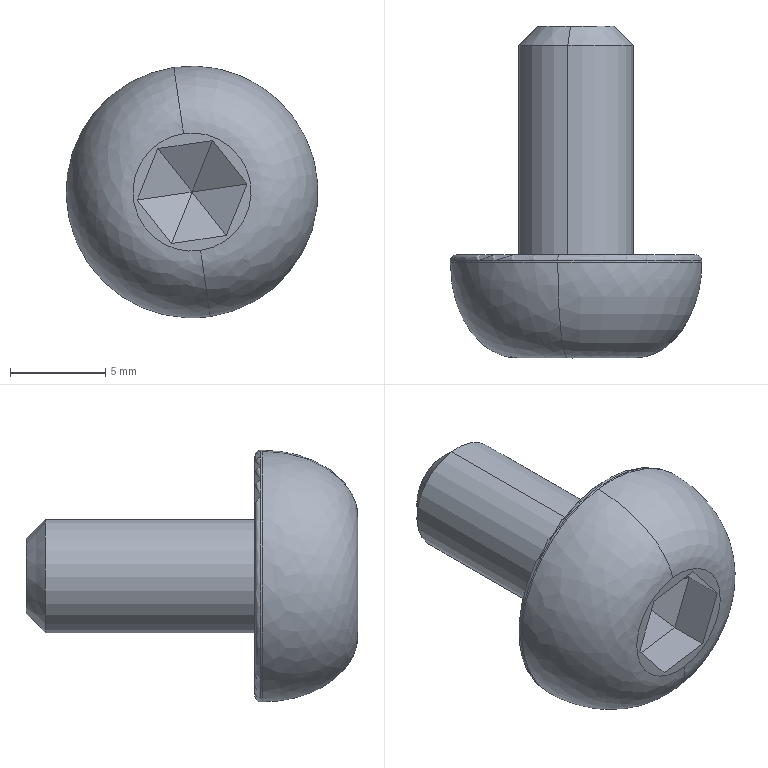Part | SolidWorks | features BaseBody 1 | 1 solid | 25 faces | box 13.2 x 17.4 x 13.2 mm | volume 875.551 mm3 | plane 15 | cylinder 4 | cone 2 | torus 2 | spline 2 | commonest cylinder face diameters 6 x2 13.2 x2
STEP:
#1=CARTESIAN_POINT('',(-484.979,-95.35,173.865));
#2=VERTEX_POINT('',#1);
#3=CARTESIAN_POINT('',(-485.556,-95.35,177.823));
#4=VERTEX_POINT('',#3);
#5=CARTESIAN_POINT('',(-485.268,-95.35,175.844));
#6=DIRECTION('',(0.,1.,0.));
#7=DIRECTION('',(0.1444,0.,-0.9895));
#8=AXIS2_PLACEMENT_3D('',#5,#6,#7);
#9=CIRCLE('',#8,2.);
#10=EDGE_CURVE('',#2,#4,#9,.T.);
#11=ORIENTED_EDGE('',*,*,#10,.F.);
#12=CARTESIAN_POINT('',(-484.835,-96.35,172.876));
#13=VERTEX_POINT('',#12);
#14=CARTESIAN_POINT('',(-484.907,-95.85,173.37));
#15=DIRECTION('',(0.1021,-0.7071,-0.6997));
#16=VECTOR('',#15,1000.);
#17=LINE('',#14,#16);
#18=EDGE_CURVE('',#2,#13,#17,.T.);
#19=ORIENTED_EDGE('',*,*,#18,.T.);
#20=CARTESIAN_POINT('',(-485.701,-96.35,178.813));
#21=VERTEX_POINT('',#20);
#22=CARTESIAN_POINT('',(-485.268,-96.35,175.844));
#23=DIRECTION('',(0.,1.,0.));
#24=DIRECTION('',(0.1444,0.,-0.9895));
#25=AXIS2_PLACEMENT_3D('',#22,#23,#24);
#26=CIRCLE('',#25,3.);
#27=EDGE_CURVE('',#13,#21,#26,.T.);
#28=ORIENTED_EDGE('',*,*,#27,.T.);
#29=CARTESIAN_POINT('',(-485.629,-95.85,178.318));
#30=DIRECTION('',(-0.1021,-0.7071,0.6997));
#31=VECTOR('',#30,1000.);
#32=LINE('',#29,#31);
#33=EDGE_CURVE('',#4,#21,#32,.T.);
#34=ORIENTED_EDGE('',*,*,#33,.F.);
#35=EDGE_LOOP('',(#11,#19,#28,#34));
#36=FACE_OUTER_BOUND('',#35,.T.);
#37=CARTESIAN_POINT('',(-485.268,-95.85,175.844));
#38=DIRECTION('',(0.,-1.,0.));
#39=DIRECTION('',(-0.1444,0.,0.9895));
#40=AXIS2_PLACEMENT_3D('',#37,#38,#39);
#41=CONICAL_SURFACE('',#40,2.5,0.7854);
#42=ADVANCED_FACE('',(#36),#41,.T.);
#43=ORIENTED_EDGE('',*,*,#27,.F.);
#44=CARTESIAN_POINT('',(-484.835,-107.35,172.876));
#45=VERTEX_POINT('',#44);
#46=CARTESIAN_POINT('',(-484.835,-95.35,172.876));
#47=DIRECTION('',(0.,-1.,0.));
#48=VECTOR('',#47,1000.);
#49=LINE('',#46,#48);
#50=EDGE_CURVE('',#13,#45,#49,.T.);
#51=ORIENTED_EDGE('',*,*,#50,.T.);
#52=CARTESIAN_POINT('',(-485.701,-107.35,178.813));
#53=VERTEX_POINT('',#52);
#54=CARTESIAN_POINT('',(-485.268,-107.35,175.844));
#55=DIRECTION('',(0.,-1.,0.));
#56=DIRECTION('',(0.1444,0.,-0.9895));
#57=AXIS2_PLACEMENT_3D('',#54,#55,#56);
#58=CIRCLE('',#57,3.);
#59=EDGE_CURVE('',#53,#45,#58,.T.);
#60=ORIENTED_EDGE('',*,*,#59,.F.);
#61=CARTESIAN_POINT('',(-485.701,-95.35,178.813));
#62=DIRECTION('',(0.,-1.,0.));
#63=VECTOR('',#62,1000.);
#64=LINE('',#61,#63);
#65=EDGE_CURVE('',#21,#53,#64,.T.);
#66=ORIENTED_EDGE('',*,*,#65,.F.);
#67=EDGE_LOOP('',(#43,#51,#60,#66));
#68=FACE_OUTER_BOUND('',#67,.T.);
#69=CARTESIAN_POINT('',(-485.268,-95.35,175.844));
#70=DIRECTION('',(0.,-1.,0.));
#71=DIRECTION('',(-0.1444,0.,0.9895));
#72=AXIS2_PLACEMENT_3D('',#69,#70,#71);
#73=CYLINDRICAL_SURFACE('',#72,3.);
#74=ADVANCED_FACE('',(#68),#73,.T.);
#75=CARTESIAN_POINT('',(-484.315,-107.65,169.313));
#76=VERTEX_POINT('',#75);
#77=CARTESIAN_POINT('',(-486.221,-107.65,182.375));
#78=VERTEX_POINT('',#77);
#79=CARTESIAN_POINT('',(-485.268,-107.65,175.844));
#80=DIRECTION('',(0.,1.,0.));
#81=DIRECTION('',(0.1444,0.,-0.9895));
#82=AXIS2_PLACEMENT_3D('',#79,#80,#81);
#83=CIRCLE('',#82,6.6);
#84=EDGE_CURVE('',#76,#78,#83,.T.);
#85=ORIENTED_EDGE('',*,*,#84,.T.);
#86=CARTESIAN_POINT('',(-486.177,-107.35,182.078));
#87=VERTEX_POINT('',#86);
#88=CARTESIAN_POINT('',(-486.177,-107.65,182.078));
#89=DIRECTION('',(-0.9895,0.,-0.1444));
#90=DIRECTION('',(-0.1444,0.,0.9895));
#91=AXIS2_PLACEMENT_3D('',#88,#89,#90);
#92=CIRCLE('',#91,0.3);
#93=EDGE_CURVE('',#78,#87,#92,.T.);
#94=ORIENTED_EDGE('',*,*,#93,.T.);
#95=CARTESIAN_POINT('',(-484.358,-107.35,169.61));
#96=VERTEX_POINT('',#95);
#97=CARTESIAN_POINT('',(-485.268,-107.35,175.844));
#98=DIRECTION('',(0.,1.,0.));
#99=DIRECTION('',(0.1444,0.,-0.9895));
#100=AXIS2_PLACEMENT_3D('',#97,#98,#99);
#101=CIRCLE('',#100,6.3);
#102=EDGE_CURVE('',#96,#87,#101,.T.);
#103=ORIENTED_EDGE('',*,*,#102,.F.);
#104=CARTESIAN_POINT('',(-484.358,-107.65,169.61));
#105=DIRECTION('',(0.9895,0.,0.1444));
#106=DIRECTION('',(0.1444,0.,-0.9895));
#107=AXIS2_PLACEMENT_3D('',#104,#105,#106);
#108=CIRCLE('',#107,0.3);
#109=EDGE_CURVE('',#76,#96,#108,.T.);
#110=ORIENTED_EDGE('',*,*,#109,.F.);
#111=EDGE_LOOP('',(#85,#94,#103,#110));
#112=FACE_OUTER_BOUND('',#111,.T.);
#113=CARTESIAN_POINT('',(-485.268,-107.65,175.844));
#114=DIRECTION('',(0.,1.,0.));
#115=DIRECTION('',(0.1444,0.,-0.9895));
#116=AXIS2_PLACEMENT_3D('',#113,#114,#115);
#117=TOROIDAL_SURFACE('',#116,6.3,0.3);
#118=ADVANCED_FACE('',(#112),#117,.T.);
#119=ORIENTED_EDGE('',*,*,#84,.F.);
#120=CARTESIAN_POINT('',(-484.315,-107.75,169.314));
#121=VERTEX_POINT('',#120);
#122=CARTESIAN_POINT('',(-484.315,-107.35,169.313));
#123=DIRECTION('',(0.,-1.,0.));
#124=VECTOR('',#123,1000.);
#125=LINE('',#122,#124);
#126=EDGE_CURVE('',#76,#121,#125,.T.);
#127=ORIENTED_EDGE('',*,*,#126,.T.);
#128=CARTESIAN_POINT('',(-486.221,-107.75,182.375));
#129=VERTEX_POINT('',#128);
#130=CARTESIAN_POINT('',(-486.221,-107.75,182.375));
#131=CARTESIAN_POINT('',(-499.282,-107.75,180.469));
#132=CARTESIAN_POINT('',(-497.376,-107.75,167.408));
#133=CARTESIAN_POINT('',(-484.315,-107.75,169.314));
#134=(BOUNDED_CURVE()B_SPLINE_CURVE(3,(#130,#131,#132,#133),.UNSPECIFIED.,.F.,.F.)B_SPLINE_CURVE_WITH_KNOTS((4,4),(0.,1.),.UNSPECIFIED.)CURVE()GEOMETRIC_REPRESENTATION_ITEM()RATIONAL_B_SPLINE_CURVE((1.,0.3333,0.3333,1.))REPRESENTATION_ITEM(''));
#135=EDGE_CURVE('',#129,#121,#134,.T.);
#136=ORIENTED_EDGE('',*,*,#135,.F.);
#137=CARTESIAN_POINT('',(-486.221,-107.35,182.375));
#138=DIRECTION('',(0.,-1.,0.));
#139=VECTOR('',#138,1000.);
#140=LINE('',#137,#139);
#141=EDGE_CURVE('',#78,#129,#140,.T.);
#142=ORIENTED_EDGE('',*,*,#141,.F.);
#143=EDGE_LOOP('',(#119,#127,#136,#142));
#144=FACE_OUTER_BOUND('',#143,.T.);
#145=CARTESIAN_POINT('',(-485.268,-107.35,175.844));
#146=DIRECTION('',(0.,-1.,0.));
#147=DIRECTION('',(-0.1444,0.,0.9895));
#148=AXIS2_PLACEMENT_3D('',#145,#146,#147);
#149=CYLINDRICAL_SURFACE('',#148,6.6);
#150=ADVANCED_FACE('',(#144),#149,.T.);
#151=CARTESIAN_POINT('',(-484.194,-110.67,178.543));
#152=VERTEX_POINT('',#151);
#153=CARTESIAN_POINT('',(-485.268,-109.218,175.844));
#154=VERTEX_POINT('',#153);
#155=CARTESIAN_POINT('',(-484.194,-110.67,178.543));
#156=DIRECTION('',(-0.3307,0.4472,-0.8311));
#157=VECTOR('',#156,1000.);
#158=LINE('',#155,#157);
#159=EDGE_CURVE('',#152,#154,#158,.T.);
#160=ORIENTED_EDGE('',*,*,#159,.T.);
#161=CARTESIAN_POINT('',(-482.394,-110.67,176.264));
#162=VERTEX_POINT('',#161);
#163=CARTESIAN_POINT('',(-482.394,-110.67,176.264));
#164=DIRECTION('',(-0.8851,0.4472,-0.1292));
#165=VECTOR('',#164,1000.);
#166=LINE('',#163,#165);
#167=EDGE_CURVE('',#162,#154,#166,.T.);
#168=ORIENTED_EDGE('',*,*,#167,.F.);
#169=CARTESIAN_POINT('',(-482.394,-110.67,176.264));
#170=DIRECTION('',(-0.6198,0.,0.7848));
#171=VECTOR('',#170,1000.);
#172=LINE('',#169,#171);
#173=EDGE_CURVE('',#162,#152,#172,.T.);
#174=ORIENTED_EDGE('',*,*,#173,.T.);
#175=EDGE_LOOP('',(#160,#168,#174));
#176=FACE_OUTER_BOUND('',#175,.T.);
#177=CARTESIAN_POINT('',(-482.394,-110.67,176.264));
#178=DIRECTION('',(0.3924,0.866,0.3099));
#179=DIRECTION('',(0.6198,0.,-0.7848));
#180=AXIS2_PLACEMENT_3D('',#177,#178,#179);
#181=PLANE('',#180);
#182=ADVANCED_FACE('',(#176),#181,.F.);
#183=CARTESIAN_POINT('',(-484.194,-112.75,178.543));
#184=VERTEX_POINT('',#183);
#185=CARTESIAN_POINT('',(-484.194,-112.75,178.543));
#186=DIRECTION('',(0.,1.,0.));
#187=VECTOR('',#186,1000.);
#188=LINE('',#185,#187);
#189=EDGE_CURVE('',#184,#152,#188,.T.);
#190=ORIENTED_EDGE('',*,*,#189,.T.);
#191=ORIENTED_EDGE('',*,*,#173,.F.);
#192=CARTESIAN_POINT('',(-482.394,-112.75,176.264));
#193=VERTEX_POINT('',#192);
#194=CARTESIAN_POINT('',(-482.394,-112.75,176.264));
#195=DIRECTION('',(0.,1.,0.));
#196=VECTOR('',#195,1000.);
#197=LINE('',#194,#196);
#198=EDGE_CURVE('',#193,#162,#197,.T.);
#199=ORIENTED_EDGE('',*,*,#198,.F.);
#200=CARTESIAN_POINT('',(-484.194,-112.75,178.543));
#201=DIRECTION('',(0.6198,0.,-0.7848));
#202=VECTOR('',#201,1000.);
#203=LINE('',#200,#202);
#204=EDGE_CURVE('',#184,#193,#203,.T.);
#205=ORIENTED_EDGE('',*,*,#204,.F.);
#206=EDGE_LOOP('',(#190,#191,#199,#205));
#207=FACE_OUTER_BOUND('',#206,.T.);
#208=CARTESIAN_POINT('',(-482.394,-110.67,176.264));
#209=DIRECTION('',(0.7848,0.,0.6198));
#210=DIRECTION('',(0.,-1.,0.));
#211=AXIS2_PLACEMENT_3D('',#208,#209,#210);
#212=PLANE('',#211);
#213=ADVANCED_FACE('',(#207),#212,.F.);
#214=CARTESIAN_POINT('',(-488.141,-112.75,175.425));
#215=VERTEX_POINT('',#214);
#216=CARTESIAN_POINT('',(-487.068,-112.75,178.123));
#217=VERTEX_POINT('',#216);
#218=CARTESIAN_POINT('',(-488.141,-112.75,175.425));
#219=DIRECTION('',(0.3697,0.,0.9291));
#220=VECTOR('',#219,1000.);
#221=LINE('',#218,#220);
#222=EDGE_CURVE('',#215,#217,#221,.T.);
#223=ORIENTED_EDGE('',*,*,#222,.T.);
#224=CARTESIAN_POINT('',(-487.068,-112.75,178.123));
#225=DIRECTION('',(0.9895,0.,0.1444));
#226=VECTOR('',#225,1000.);
#227=LINE('',#224,#226);
#228=EDGE_CURVE('',#217,#184,#227,.T.);
#229=ORIENTED_EDGE('',*,*,#228,.T.);
#230=ORIENTED_EDGE('',*,*,#204,.T.);
#231=CARTESIAN_POINT('',(-483.468,-112.75,173.565));
#232=VERTEX_POINT('',#231);
#233=CARTESIAN_POINT('',(-482.394,-112.75,176.264));
#234=DIRECTION('',(-0.3697,0.,-0.9291));
#235=VECTOR('',#234,1000.);
#236=LINE('',#233,#235);
#237=EDGE_CURVE('',#193,#232,#236,.T.);
#238=ORIENTED_EDGE('',*,*,#237,.T.);
#239=CARTESIAN_POINT('',(-486.341,-112.75,173.146));
#240=VERTEX_POINT('',#239);
#241=CARTESIAN_POINT('',(-483.468,-112.75,173.565));
#242=DIRECTION('',(-0.9895,0.,-0.1444));
#243=VECTOR('',#242,1000.);
#244=LINE('',#241,#243);
#245=EDGE_CURVE('',#232,#240,#244,.T.);
#246=ORIENTED_EDGE('',*,*,#245,.T.);
#247=CARTESIAN_POINT('',(-486.341,-112.75,173.146));
#248=DIRECTION('',(-0.6198,0.,0.7848));
#249=VECTOR('',#248,1000.);
#250=LINE('',#247,#249);
#251=EDGE_CURVE('',#240,#215,#250,.T.);
#252=ORIENTED_EDGE('',*,*,#251,.T.);
#253=EDGE_LOOP('',(#223,#229,#230,#238,#246,#252));
#254=FACE_BOUND('',#253,.T.);
#255=CARTESIAN_POINT('',(-484.82,-112.75,172.777));
#256=VERTEX_POINT('',#255);
#257=CARTESIAN_POINT('',(-485.715,-112.75,178.912));
#258=VERTEX_POINT('',#257);
#259=CARTESIAN_POINT('',(-484.82,-112.75,172.777));
#260=CARTESIAN_POINT('',(-484.72,-112.75,172.791));
#261=CARTESIAN_POINT('',(-484.621,-112.75,172.811));
#262=CARTESIAN_POINT('',(-484.425,-112.75,172.86));
#263=CARTESIAN_POINT('',(-484.325,-112.75,172.89));
#264=CARTESIAN_POINT('',(-484.04,-112.75,172.993));
#265=CARTESIAN_POINT('',(-483.856,-112.75,173.08));
#266=CARTESIAN_POINT('',(-483.507,-112.75,173.288));
#267=CARTESIAN_POINT('',(-483.345,-112.75,173.407));
#268=CARTESIAN_POINT('',(-483.04,-112.75,173.68));
#269=CARTESIAN_POINT('',(-482.902,-112.75,173.83));
#270=CARTESIAN_POINT('',(-482.722,-112.75,174.072));
#271=CARTESIAN_POINT('',(-482.666,-112.75,174.156));
#272=CARTESIAN_POINT('',(-482.562,-112.75,174.33));
#273=CARTESIAN_POINT('',(-482.513,-112.75,174.422));
#274=CARTESIAN_POINT('',(-482.384,-112.75,174.696));
#275=CARTESIAN_POINT('',(-482.315,-112.75,174.888));
#276=CARTESIAN_POINT('',(-482.215,-112.75,175.282));
#277=CARTESIAN_POINT('',(-482.185,-112.75,175.481));
#278=CARTESIAN_POINT('',(-482.162,-112.75,175.889));
#279=CARTESIAN_POINT('',(-482.171,-112.75,176.093));
#280=CARTESIAN_POINT('',(-482.215,-112.75,176.391));
#281=CARTESIAN_POINT('',(-482.234,-112.75,176.49));
#282=CARTESIAN_POINT('',(-482.283,-112.75,176.687));
#283=CARTESIAN_POINT('',(-482.314,-112.75,176.786));
#284=CARTESIAN_POINT('',(-482.416,-112.75,177.071));
#285=CARTESIAN_POINT('',(-482.503,-112.75,177.256));
#286=CARTESIAN_POINT('',(-482.711,-112.75,177.605));
#287=CARTESIAN_POINT('',(-482.831,-112.75,177.767));
#288=CARTESIAN_POINT('',(-483.103,-112.75,178.072));
#289=CARTESIAN_POINT('',(-483.254,-112.75,178.209));
#290=CARTESIAN_POINT('',(-483.496,-112.75,178.39));
#291=CARTESIAN_POINT('',(-483.58,-112.75,178.446));
#292=CARTESIAN_POINT('',(-483.753,-112.75,178.55));
#293=CARTESIAN_POINT('',(-483.845,-112.75,178.599));
#294=CARTESIAN_POINT('',(-484.119,-112.75,178.729));
#295=CARTESIAN_POINT('',(-484.31,-112.75,178.797));
#296=CARTESIAN_POINT('',(-484.704,-112.75,178.897));
#297=CARTESIAN_POINT('',(-484.903,-112.75,178.928));
#298=CARTESIAN_POINT('',(-485.312,-112.75,178.95));
#299=CARTESIAN_POINT('',(-485.515,-112.75,178.941));
#300=CARTESIAN_POINT('',(-485.715,-112.75,178.912));
#301=B_SPLINE_CURVE_WITH_KNOTS('',3,(#259,#260,#261,#262,#263,#264,#265,#266,#267,#268,#269,#270,#271,#272,#273,#274,#275,#276,#277,#278,#279,#280,#281,#282,#283,#284,#285,#286,#287,#288,#289,#290,#291,#292,#293,#294,#295,#296,#297,#298,#299,#300),.UNSPECIFIED.,.F.,.F.,(4,2,2,2,2,2,2,2,2,2,2,2,2,2,2,2,2,2,2,2,4),(0.,0.03125,0.0625,0.125,0.1875,0.25,0.2812,0.3125,0.375,0.4375,0.5,0.5313,0.5625,0.625,0.6875,0.75,0.7813,0.8125,0.875,0.9375,1.),.UNSPECIFIED.);
#302=EDGE_CURVE('',#256,#258,#301,.T.);
#303=ORIENTED_EDGE('',*,*,#302,.T.);
#304=CARTESIAN_POINT('',(-485.715,-112.75,178.912));
#305=CARTESIAN_POINT('',(-485.815,-112.75,178.897));
#306=CARTESIAN_POINT('',(-485.914,-112.75,178.878));
#307=CARTESIAN_POINT('',(-486.111,-112.75,178.828));
#308=CARTESIAN_POINT('',(-486.21,-112.75,178.798));
#309=CARTESIAN_POINT('',(-486.495,-112.75,178.696));
#310=CARTESIAN_POINT('',(-486.679,-112.75,178.609));
#311=CARTESIAN_POINT('',(-487.029,-112.75,178.401));
#312=CARTESIAN_POINT('',(-487.191,-112.75,178.281));
#313=CARTESIAN_POINT('',(-487.495,-112.75,178.009));
#314=CARTESIAN_POINT('',(-487.633,-112.75,177.858));
#315=CARTESIAN_POINT('',(-487.813,-112.75,177.616));
#316=CARTESIAN_POINT('',(-487.87,-112.75,177.532));
#317=CARTESIAN_POINT('',(-487.974,-112.75,177.359));
#318=CARTESIAN_POINT('',(-488.023,-112.75,177.267));
#319=CARTESIAN_POINT('',(-488.152,-112.75,176.993));
#320=CARTESIAN_POINT('',(-488.22,-112.75,176.801));
#321=CARTESIAN_POINT('',(-488.32,-112.75,176.407));
#322=CARTESIAN_POINT('',(-488.351,-112.75,176.208));
#323=CARTESIAN_POINT('',(-488.373,-112.75,175.8));
#324=CARTESIAN_POINT('',(-488.364,-112.75,175.596));
#325=CARTESIAN_POINT('',(-488.321,-112.75,175.297));
#326=CARTESIAN_POINT('',(-488.301,-112.75,175.198));
#327=CARTESIAN_POINT('',(-488.252,-112.75,175.002));
#328=CARTESIAN_POINT('',(-488.222,-112.75,174.902));
#329=CARTESIAN_POINT('',(-488.119,-112.75,174.617));
#330=CARTESIAN_POINT('',(-488.032,-112.75,174.433));
#331=CARTESIAN_POINT('',(-487.824,-112.75,174.084));
#332=CARTESIAN_POINT('',(-487.705,-112.75,173.921));
#333=CARTESIAN_POINT('',(-487.432,-112.75,173.617));
#334=CARTESIAN_POINT('',(-487.282,-112.75,173.479));
#335=CARTESIAN_POINT('',(-487.04,-112.75,173.299));
#336=CARTESIAN_POINT('',(-486.956,-112.75,173.242));
#337=CARTESIAN_POINT('',(-486.782,-112.75,173.138));
#338=CARTESIAN_POINT('',(-486.691,-112.75,173.089));
#339=CARTESIAN_POINT('',(-486.417,-112.75,172.96));
#340=CARTESIAN_POINT('',(-486.225,-112.75,172.891));
#341=CARTESIAN_POINT('',(-485.831,-112.75,172.792));
#342=CARTESIAN_POINT('',(-485.633,-112.75,172.761));
#343=CARTESIAN_POINT('',(-485.223,-112.75,172.738));
#344=CARTESIAN_POINT('',(-485.021,-112.75,172.747));
#345=CARTESIAN_POINT('',(-484.82,-112.75,172.777));
#346=B_SPLINE_CURVE_WITH_KNOTS('',3,(#304,#305,#306,#307,#308,#309,#310,#311,#312,#313,#314,#315,#316,#317,#318,#319,#320,#321,#322,#323,#324,#325,#326,#327,#328,#329,#330,#331,#332,#333,#334,#335,#336,#337,#338,#339,#340,#341,#342,#343,#344,#345),.UNSPECIFIED.,.F.,.F.,(4,2,2,2,2,2,2,2,2,2,2,2,2,2,2,2,2,2,2,2,4),(0.,0.03125,0.0625,0.125,0.1875,0.25,0.2813,0.3125,0.375,0.4375,0.5,0.5313,0.5625,0.625,0.6875,0.75,0.7813,0.8125,0.875,0.9375,1.),.UNSPECIFIED.);
#347=EDGE_CURVE('',#258,#256,#346,.T.);
#348=ORIENTED_EDGE('',*,*,#347,.T.);
#349=EDGE_LOOP('',(#303,#348));
#350=FACE_OUTER_BOUND('',#349,.T.);
#351=CARTESIAN_POINT('',(-485.268,-112.75,175.844));
#352=DIRECTION('',(0.,1.,0.));
#353=DIRECTION('',(1.,0.,0.));
#354=AXIS2_PLACEMENT_3D('',#351,#352,#353);
#355=PLANE('',#354);
#356=ADVANCED_FACE('',(#254,#350),#355,.F.);
#357=CARTESIAN_POINT('',(-484.315,-107.75,169.314));
#358=CARTESIAN_POINT('',(-484.315,-108.331,169.314));
#359=CARTESIAN_POINT('',(-484.331,-109.281,169.424));
#360=CARTESIAN_POINT('',(-484.393,-110.497,169.853));
#361=CARTESIAN_POINT('',(-484.461,-111.324,170.318));
#362=CARTESIAN_POINT('',(-484.545,-111.99,170.893));
#363=CARTESIAN_POINT('',(-484.667,-112.596,171.731));
#364=CARTESIAN_POINT('',(-484.762,-112.75,172.381));
#365=CARTESIAN_POINT('',(-484.82,-112.75,172.777));
#366=(BOUNDED_CURVE()B_SPLINE_CURVE(3,(#357,#358,#359,#360,#361,#362,#363,#364,#365),.UNSPECIFIED.,.F.,.T.)B_SPLINE_CURVE_WITH_KNOTS((4,1,1,1,1,1,4),(0.,0.2462,0.3741,0.502,0.6299,0.7578,1.),.UNSPECIFIED.)CURVE()GEOMETRIC_REPRESENTATION_ITEM()RATIONAL_B_SPLINE_CURVE((1.,1.,1.,1.,1.,1.,1.,1.,1.))REPRESENTATION_ITEM(''));
#367=EDGE_CURVE('',#121,#256,#366,.T.);
#368=ORIENTED_EDGE('',*,*,#367,.T.);
#369=ORIENTED_EDGE('',*,*,#347,.F.);
#370=CARTESIAN_POINT('',(-486.221,-107.75,182.375));
#371=CARTESIAN_POINT('',(-486.221,-108.331,182.375));
#372=CARTESIAN_POINT('',(-486.205,-109.281,182.265));
#373=CARTESIAN_POINT('',(-486.142,-110.497,181.836));
#374=CARTESIAN_POINT('',(-486.074,-111.324,181.371));
#375=CARTESIAN_POINT('',(-485.99,-111.99,180.795));
#376=CARTESIAN_POINT('',(-485.868,-112.596,179.958));
#377=CARTESIAN_POINT('',(-485.773,-112.75,179.308));
#378=CARTESIAN_POINT('',(-485.715,-112.75,178.912));
#379=B_SPLINE_CURVE_WITH_KNOTS('',3,(#370,#371,#372,#373,#374,#375,#376,#377,#378),.UNSPECIFIED.,.F.,.F.,(4,1,1,1,1,1,4),(0.,0.2462,0.3741,0.502,0.6299,0.7578,1.),.UNSPECIFIED.);
#380=EDGE_CURVE('',#129,#258,#379,.T.);
#381=ORIENTED_EDGE('',*,*,#380,.F.);
#382=ORIENTED_EDGE('',*,*,#135,.T.);
#383=EDGE_LOOP('',(#368,#369,#381,#382));
#384=FACE_OUTER_BOUND('',#383,.T.);
#385=CARTESIAN_POINT('',(-486.221,-107.75,182.375));
#386=CARTESIAN_POINT('',(-499.282,-107.75,180.469));
#387=CARTESIAN_POINT('',(-497.376,-107.75,167.408));
#388=CARTESIAN_POINT('',(-484.315,-107.75,169.314));
#389=CARTESIAN_POINT('',(-486.221,-108.331,182.375));
#390=CARTESIAN_POINT('',(-499.282,-108.331,180.469));
#391=CARTESIAN_POINT('',(-497.376,-108.331,167.408));
#392=CARTESIAN_POINT('',(-484.315,-108.331,169.314));
#393=CARTESIAN_POINT('',(-486.205,-109.281,182.265));
#394=CARTESIAN_POINT('',(-499.046,-109.281,180.391));
#395=CARTESIAN_POINT('',(-497.172,-109.281,167.55));
#396=CARTESIAN_POINT('',(-484.331,-109.281,169.424));
#397=CARTESIAN_POINT('',(-486.142,-110.497,181.836));
#398=CARTESIAN_POINT('',(-498.126,-110.497,180.087));
#399=CARTESIAN_POINT('',(-496.377,-110.497,168.104));
#400=CARTESIAN_POINT('',(-484.393,-110.497,169.853));
#401=CARTESIAN_POINT('',(-486.074,-111.324,181.371));
#402=CARTESIAN_POINT('',(-497.127,-111.324,179.758));
#403=CARTESIAN_POINT('',(-495.514,-111.324,168.705));
#404=CARTESIAN_POINT('',(-484.461,-111.324,170.318));
#405=CARTESIAN_POINT('',(-485.99,-111.99,180.795));
#406=CARTESIAN_POINT('',(-495.892,-111.99,179.35));
#407=CARTESIAN_POINT('',(-494.447,-111.99,169.449));
#408=CARTESIAN_POINT('',(-484.545,-111.99,170.893));
#409=CARTESIAN_POINT('',(-485.866,-112.604,179.947));
#410=CARTESIAN_POINT('',(-494.071,-112.604,178.749));
#411=CARTESIAN_POINT('',(-492.874,-112.604,170.544));
#412=CARTESIAN_POINT('',(-484.669,-112.604,171.742));
#413=CARTESIAN_POINT('',(-485.77,-112.755,179.284));
#414=CARTESIAN_POINT('',(-492.65,-112.755,178.28));
#415=CARTESIAN_POINT('',(-491.646,-112.755,171.4));
#416=CARTESIAN_POINT('',(-484.766,-112.755,172.404));
#417=CARTESIAN_POINT('',(-485.711,-112.75,178.88));
#418=CARTESIAN_POINT('',(-491.782,-112.75,177.994));
#419=CARTESIAN_POINT('',(-490.896,-112.75,171.923));
#420=CARTESIAN_POINT('',(-484.825,-112.75,172.809));
#421=(BOUNDED_SURFACE()B_SPLINE_SURFACE(3,3,((#385,#386,#387,#388),(#389,#390,#391,#392),(#393,#394,#395,#396),(#397,#398,#399,#400),(#401,#402,#403,#404),(#405,#406,#407,#408),(#409,#410,#411,#412),(#413,#414,#415,#416),(#417,#418,#419,#420)),.UNSPECIFIED.,.F.,.F.,.T.)B_SPLINE_SURFACE_WITH_KNOTS((4,1,1,1,1,1,4),(4,4),(0.009324,0.25,0.375,0.5,0.625,0.75,0.9931),(0.,1.),.UNSPECIFIED.)GEOMETRIC_REPRESENTATION_ITEM()RATIONAL_B_SPLINE_SURFACE(((1.,0.3333,0.3333,1.),(1.,0.3333,0.3333,1.),(1.,0.3333,0.3333,1.),(1.,0.3333,0.3333,1.),(1.,0.3333,0.3333,1.),(1.,0.3333,0.3333,1.),(1.,0.3333,0.3333,1.),(1.,0.3333,0.3333,1.),(1.,0.3333,0.3333,1.)))REPRESENTATION_ITEM('')SURFACE());
#422=ADVANCED_FACE('',(#384),#421,.F.);
#423=ORIENTED_EDGE('',*,*,#126,.F.);
#424=CARTESIAN_POINT('',(-485.268,-107.65,175.844));
#425=DIRECTION('',(0.,1.,0.));
#426=DIRECTION('',(0.1444,0.,-0.9895));
#427=AXIS2_PLACEMENT_3D('',#424,#425,#426);
#428=CIRCLE('',#427,6.6);
#429=EDGE_CURVE('',#78,#76,#428,.T.);
#430=ORIENTED_EDGE('',*,*,#429,.F.);
#431=ORIENTED_EDGE('',*,*,#141,.T.);
#432=CARTESIAN_POINT('',(-484.315,-107.75,169.314));
#433=CARTESIAN_POINT('',(-480.489,-107.75,169.872));
#434=CARTESIAN_POINT('',(-478.179,-107.75,172.972));
#435=CARTESIAN_POINT('',(-478.737,-107.75,176.797));
#436=CARTESIAN_POINT('',(-479.295,-107.75,180.623));
#437=CARTESIAN_POINT('',(-482.395,-107.75,182.933));
#438=CARTESIAN_POINT('',(-486.221,-107.75,182.375));
#439=(BOUNDED_CURVE()B_SPLINE_CURVE(3,(#432,#433,#434,#435,#436,#437,#438),.UNSPECIFIED.,.F.,.T.)B_SPLINE_CURVE_WITH_KNOTS((4,3,4),(0.,0.5,1.),.UNSPECIFIED.)CURVE()GEOMETRIC_REPRESENTATION_ITEM()RATIONAL_B_SPLINE_CURVE((1.,0.8047,0.8047,1.,0.8047,0.8047,1.))REPRESENTATION_ITEM(''));
#440=EDGE_CURVE('',#121,#129,#439,.T.);
#441=ORIENTED_EDGE('',*,*,#440,.F.);
#442=EDGE_LOOP('',(#423,#430,#431,#441));
#443=FACE_OUTER_BOUND('',#442,.T.);
#444=CARTESIAN_POINT('',(-485.268,-107.35,175.844));
#445=DIRECTION('',(0.,-1.,0.));
#446=DIRECTION('',(-0.1444,0.,0.9895));
#447=AXIS2_PLACEMENT_3D('',#444,#445,#446);
#448=CYLINDRICAL_SURFACE('',#447,6.6);
#449=ADVANCED_FACE('',(#443),#448,.T.);
#450=ORIENTED_EDGE('',*,*,#93,.F.);
#451=ORIENTED_EDGE('',*,*,#429,.T.);
#452=ORIENTED_EDGE('',*,*,#109,.T.);
#453=CARTESIAN_POINT('',(-485.268,-107.35,175.844));
#454=DIRECTION('',(0.,1.,0.));
#455=DIRECTION('',(0.1444,0.,-0.9895));
#456=AXIS2_PLACEMENT_3D('',#453,#454,#455);
#457=CIRCLE('',#456,6.3);
#458=EDGE_CURVE('',#87,#96,#457,.T.);
#459=ORIENTED_EDGE('',*,*,#458,.F.);
#460=EDGE_LOOP('',(#450,#451,#452,#459));
#461=FACE_OUTER_BOUND('',#460,.T.);
#462=CARTESIAN_POINT('',(-485.268,-107.65,175.844));
#463=DIRECTION('',(0.,1.,0.));
#464=DIRECTION('',(0.1444,0.,-0.9895));
#465=AXIS2_PLACEMENT_3D('',#462,#463,#464);
#466=TOROIDAL_SURFACE('',#465,6.3,0.3);
#467=ADVANCED_FACE('',(#461),#466,.T.);
#468=ORIENTED_EDGE('',*,*,#59,.T.);
#469=CARTESIAN_POINT('',(-485.268,-107.35,175.844));
#470=DIRECTION('',(0.,-1.,0.));
#471=DIRECTION('',(0.1444,0.,-0.9895));
#472=AXIS2_PLACEMENT_3D('',#469,#470,#471);
#473=CIRCLE('',#472,3.);
#474=EDGE_CURVE('',#45,#53,#473,.T.);
#475=ORIENTED_EDGE('',*,*,#474,.T.);
#476=EDGE_LOOP('',(#468,#475));
#477=FACE_BOUND('',#476,.T.);
#478=ORIENTED_EDGE('',*,*,#102,.T.);
#479=ORIENTED_EDGE('',*,*,#458,.T.);
#480=EDGE_LOOP('',(#478,#479));
#481=FACE_OUTER_BOUND('',#480,.T.);
#482=CARTESIAN_POINT('',(-485.268,-107.35,175.844));
#483=DIRECTION('',(0.,1.,0.));
#484=DIRECTION('',(1.,0.,0.));
#485=AXIS2_PLACEMENT_3D('',#482,#483,#484);
#486=PLANE('',#485);
#487=ADVANCED_FACE('',(#477,#481),#486,.T.);
#488=ORIENTED_EDGE('',*,*,#50,.F.);
#489=CARTESIAN_POINT('',(-485.268,-96.35,175.844));
#490=DIRECTION('',(0.,1.,0.));
#491=DIRECTION('',(0.1444,0.,-0.9895));
#492=AXIS2_PLACEMENT_3D('',#489,#490,#491);
#493=CIRCLE('',#492,3.);
#494=EDGE_CURVE('',#21,#13,#493,.T.);
#495=ORIENTED_EDGE('',*,*,#494,.F.);
#496=ORIENTED_EDGE('',*,*,#65,.T.);
#497=ORIENTED_EDGE('',*,*,#474,.F.);
#498=EDGE_LOOP('',(#488,#495,#496,#497));
#499=FACE_OUTER_BOUND('',#498,.T.);
#500=CARTESIAN_POINT('',(-485.268,-95.35,175.844));
#501=DIRECTION('',(0.,-1.,0.));
#502=DIRECTION('',(-0.1444,0.,0.9895));
#503=AXIS2_PLACEMENT_3D('',#500,#501,#502);
#504=CYLINDRICAL_SURFACE('',#503,3.);
#505=ADVANCED_FACE('',(#499),#504,.T.);
#506=CARTESIAN_POINT('',(-485.268,-95.35,175.844));
#507=DIRECTION('',(0.,1.,0.));
#508=DIRECTION('',(0.1444,0.,-0.9895));
#509=AXIS2_PLACEMENT_3D('',#506,#507,#508);
#510=CIRCLE('',#509,2.);
#511=EDGE_CURVE('',#4,#2,#510,.T.);
#512=ORIENTED_EDGE('',*,*,#511,.T.);
#513=ORIENTED_EDGE('',*,*,#10,.T.);
#514=EDGE_LOOP('',(#512,#513));
#515=FACE_OUTER_BOUND('',#514,.T.);
#516=CARTESIAN_POINT('',(-485.268,-95.35,175.844));
#517=DIRECTION('',(0.,1.,0.));
#518=DIRECTION('',(1.,0.,0.));
#519=AXIS2_PLACEMENT_3D('',#516,#517,#518);
#520=PLANE('',#519);
#521=ADVANCED_FACE('',(#515),#520,.T.);
#522=ORIENTED_EDGE('',*,*,#18,.F.);
#523=ORIENTED_EDGE('',*,*,#511,.F.);
#524=ORIENTED_EDGE('',*,*,#33,.T.);
#525=ORIENTED_EDGE('',*,*,#494,.T.);
#526=EDGE_LOOP('',(#522,#523,#524,#525));
#527=FACE_OUTER_BOUND('',#526,.T.);
#528=CARTESIAN_POINT('',(-485.268,-95.85,175.844));
#529=DIRECTION('',(0.,-1.,0.));
#530=DIRECTION('',(-0.1444,0.,0.9895));
#531=AXIS2_PLACEMENT_3D('',#528,#529,#530);
#532=CONICAL_SURFACE('',#531,2.5,0.7854);
#533=ADVANCED_FACE('',(#527),#532,.T.);
#534=ORIENTED_EDGE('',*,*,#440,.T.);
#535=ORIENTED_EDGE('',*,*,#380,.T.);
#536=ORIENTED_EDGE('',*,*,#302,.F.);
#537=ORIENTED_EDGE('',*,*,#367,.F.);
#538=EDGE_LOOP('',(#534,#535,#536,#537));
#539=FACE_OUTER_BOUND('',#538,.T.);
#540=CARTESIAN_POINT('',(-484.315,-107.75,169.314));
#541=CARTESIAN_POINT('',(-480.489,-107.75,169.872));
#542=CARTESIAN_POINT('',(-478.179,-107.75,172.972));
#543=CARTESIAN_POINT('',(-478.737,-107.75,176.797));
#544=CARTESIAN_POINT('',(-479.295,-107.75,180.623));
#545=CARTESIAN_POINT('',(-482.395,-107.75,182.933));
#546=CARTESIAN_POINT('',(-486.221,-107.75,182.375));
#547=CARTESIAN_POINT('',(-484.315,-108.331,169.314));
#548=CARTESIAN_POINT('',(-480.489,-108.331,169.872));
#549=CARTESIAN_POINT('',(-478.179,-108.331,172.972));
#550=CARTESIAN_POINT('',(-478.737,-108.331,176.797));
#551=CARTESIAN_POINT('',(-479.295,-108.331,180.623));
#552=CARTESIAN_POINT('',(-482.395,-108.331,182.933));
#553=CARTESIAN_POINT('',(-486.221,-108.331,182.375));
#554=CARTESIAN_POINT('',(-484.331,-109.281,169.424));
#555=CARTESIAN_POINT('',(-480.57,-109.281,169.972));
#556=CARTESIAN_POINT('',(-478.298,-109.281,173.02));
#557=CARTESIAN_POINT('',(-478.847,-109.281,176.781));
#558=CARTESIAN_POINT('',(-479.396,-109.281,180.542));
#559=CARTESIAN_POINT('',(-482.443,-109.281,182.814));
#560=CARTESIAN_POINT('',(-486.205,-109.281,182.265));
#561=CARTESIAN_POINT('',(-484.393,-110.497,169.853));
#562=CARTESIAN_POINT('',(-480.883,-110.497,170.365));
#563=CARTESIAN_POINT('',(-478.764,-110.497,173.209));
#564=CARTESIAN_POINT('',(-479.276,-110.497,176.719));
#565=CARTESIAN_POINT('',(-479.788,-110.497,180.229));
#566=CARTESIAN_POINT('',(-482.632,-110.497,182.348));
#567=CARTESIAN_POINT('',(-486.142,-110.497,181.836));
#568=CARTESIAN_POINT('',(-484.461,-111.324,170.318));
#569=CARTESIAN_POINT('',(-481.224,-111.324,170.79));
#570=CARTESIAN_POINT('',(-479.269,-111.324,173.413));
#571=CARTESIAN_POINT('',(-479.741,-111.324,176.651));
#572=CARTESIAN_POINT('',(-480.214,-111.324,179.888));
#573=CARTESIAN_POINT('',(-482.837,-111.324,181.843));
#574=CARTESIAN_POINT('',(-486.074,-111.324,181.371));
#575=CARTESIAN_POINT('',(-484.545,-111.99,170.893));
#576=CARTESIAN_POINT('',(-481.645,-111.99,171.317));
#577=CARTESIAN_POINT('',(-479.894,-111.99,173.667));
#578=CARTESIAN_POINT('',(-480.317,-111.99,176.567));
#579=CARTESIAN_POINT('',(-480.74,-111.99,179.467));
#580=CARTESIAN_POINT('',(-483.09,-111.99,181.218));
#581=CARTESIAN_POINT('',(-485.99,-111.99,180.795));
#582=CARTESIAN_POINT('',(-484.669,-112.604,171.742));
#583=CARTESIAN_POINT('',(-482.266,-112.604,172.092));
#584=CARTESIAN_POINT('',(-480.814,-112.604,174.04));
#585=CARTESIAN_POINT('',(-481.165,-112.604,176.443));
#586=CARTESIAN_POINT('',(-481.516,-112.604,178.846));
#587=CARTESIAN_POINT('',(-483.463,-112.604,180.297));
#588=CARTESIAN_POINT('',(-485.866,-112.604,179.947));
#589=CARTESIAN_POINT('',(-484.766,-112.755,172.404));
#590=CARTESIAN_POINT('',(-482.751,-112.755,172.698));
#591=CARTESIAN_POINT('',(-481.533,-112.755,174.331));
#592=CARTESIAN_POINT('',(-481.828,-112.755,176.346));
#593=CARTESIAN_POINT('',(-482.122,-112.755,178.361));
#594=CARTESIAN_POINT('',(-483.755,-112.755,179.579));
#595=CARTESIAN_POINT('',(-485.77,-112.755,179.284));
#596=CARTESIAN_POINT('',(-484.825,-112.75,172.809));
#597=CARTESIAN_POINT('',(-483.047,-112.75,173.068));
#598=CARTESIAN_POINT('',(-481.973,-112.75,174.509));
#599=CARTESIAN_POINT('',(-482.232,-112.75,176.287));
#600=CARTESIAN_POINT('',(-482.492,-112.75,178.065));
#601=CARTESIAN_POINT('',(-483.933,-112.75,179.139));
#602=CARTESIAN_POINT('',(-485.711,-112.75,178.88));
#603=(BOUNDED_SURFACE()B_SPLINE_SURFACE(3,3,((#540,#541,#542,#543,#544,#545,#546),(#547,#548,#549,#550,#551,#552,#553),(#554,#555,#556,#557,#558,#559,#560),(#561,#562,#563,#564,#565,#566,#567),(#568,#569,#570,#571,#572,#573,#574),(#575,#576,#577,#578,#579,#580,#581),(#582,#583,#584,#585,#586,#587,#588),(#589,#590,#591,#592,#593,#594,#595),(#596,#597,#598,#599,#600,#601,#602)),.UNSPECIFIED.,.F.,.F.,.T.)B_SPLINE_SURFACE_WITH_KNOTS((4,1,1,1,1,1,4),(4,3,4),(0.009324,0.25,0.375,0.5,0.625,0.75,0.9931),(0.,0.5,1.),.UNSPECIFIED.)GEOMETRIC_REPRESENTATION_ITEM()RATIONAL_B_SPLINE_SURFACE(((1.,0.8047,0.8047,1.,0.8047,0.8047,1.),(1.,0.8047,0.8047,1.,0.8047,0.8047,1.),(1.,0.8047,0.8047,1.,0.8047,0.8047,1.),(1.,0.8047,0.8047,1.,0.8047,0.8047,1.),(1.,0.8047,0.8047,1.,0.8047,0.8047,1.),(1.,0.8047,0.8047,1.,0.8047,0.8047,1.),(1.,0.8047,0.8047,1.,0.8047,0.8047,1.),(1.,0.8047,0.8047,1.,0.8047,0.8047,1.),(1.,0.8047,0.8047,1.,0.8047,0.8047,1.)))REPRESENTATION_ITEM('')SURFACE());
#604=ADVANCED_FACE('',(#539),#603,.F.);
#605=CARTESIAN_POINT('',(-486.341,-110.67,173.146));
#606=VERTEX_POINT('',#605);
#607=CARTESIAN_POINT('',(-486.341,-112.75,173.146));
#608=DIRECTION('',(0.,1.,0.));
#609=VECTOR('',#608,1000.);
#610=LINE('',#607,#609);
#611=EDGE_CURVE('',#240,#606,#610,.T.);
#612=ORIENTED_EDGE('',*,*,#611,.T.);
#613=CARTESIAN_POINT('',(-488.141,-110.67,175.425));
#614=VERTEX_POINT('',#613);
#615=CARTESIAN_POINT('',(-488.141,-110.67,175.425));
#616=DIRECTION('',(0.6198,0.,-0.7848));
#617=VECTOR('',#616,1000.);
#618=LINE('',#615,#617);
#619=EDGE_CURVE('',#614,#606,#618,.T.);
#620=ORIENTED_EDGE('',*,*,#619,.F.);
#621=CARTESIAN_POINT('',(-488.141,-112.75,175.425));
#622=DIRECTION('',(0.,1.,0.));
#623=VECTOR('',#622,1000.);
#624=LINE('',#621,#623);
#625=EDGE_CURVE('',#215,#614,#624,.T.);
#626=ORIENTED_EDGE('',*,*,#625,.F.);
#627=ORIENTED_EDGE('',*,*,#251,.F.);
#628=EDGE_LOOP('',(#612,#620,#626,#627));
#629=FACE_OUTER_BOUND('',#628,.T.);
#630=CARTESIAN_POINT('',(-488.141,-110.67,175.425));
#631=DIRECTION('',(-0.7848,0.,-0.6198));
#632=DIRECTION('',(-0.6198,0.,0.7848));
#633=AXIS2_PLACEMENT_3D('',#630,#631,#632);
#634=PLANE('',#633);
#635=ADVANCED_FACE('',(#629),#634,.F.);
#636=ORIENTED_EDGE('',*,*,#625,.T.);
#637=CARTESIAN_POINT('',(-487.068,-110.67,178.123));
#638=VERTEX_POINT('',#637);
#639=CARTESIAN_POINT('',(-487.068,-110.67,178.123));
#640=DIRECTION('',(-0.3697,0.,-0.9291));
#641=VECTOR('',#640,1000.);
#642=LINE('',#639,#641);
#643=EDGE_CURVE('',#638,#614,#642,.T.);
#644=ORIENTED_EDGE('',*,*,#643,.F.);
#645=CARTESIAN_POINT('',(-487.068,-112.75,178.123));
#646=DIRECTION('',(0.,1.,0.));
#647=VECTOR('',#646,1000.);
#648=LINE('',#645,#647);
#649=EDGE_CURVE('',#217,#638,#648,.T.);
#650=ORIENTED_EDGE('',*,*,#649,.F.);
#651=ORIENTED_EDGE('',*,*,#222,.F.);
#652=EDGE_LOOP('',(#636,#644,#650,#651));
#653=FACE_OUTER_BOUND('',#652,.T.);
#654=CARTESIAN_POINT('',(-487.068,-110.67,178.123));
#655=DIRECTION('',(-0.9291,0.,0.3697));
#656=DIRECTION('',(0.,1.,0.));
#657=AXIS2_PLACEMENT_3D('',#654,#655,#656);
#658=PLANE('',#657);
#659=ADVANCED_FACE('',(#653),#658,.F.);
#660=ORIENTED_EDGE('',*,*,#649,.T.);
#661=CARTESIAN_POINT('',(-487.068,-110.67,178.123));
#662=DIRECTION('',(0.9895,0.,0.1444));
#663=VECTOR('',#662,1000.);
#664=LINE('',#661,#663);
#665=EDGE_CURVE('',#638,#152,#664,.T.);
#666=ORIENTED_EDGE('',*,*,#665,.T.);
#667=ORIENTED_EDGE('',*,*,#189,.F.);
#668=ORIENTED_EDGE('',*,*,#228,.F.);
#669=EDGE_LOOP('',(#660,#666,#667,#668));
#670=FACE_OUTER_BOUND('',#669,.T.);
#671=CARTESIAN_POINT('',(-484.194,-110.67,178.543));
#672=DIRECTION('',(-0.1444,0.,0.9895));
#673=DIRECTION('',(0.,1.,0.));
#674=AXIS2_PLACEMENT_3D('',#671,#672,#673);
#675=PLANE('',#674);
#676=ADVANCED_FACE('',(#670),#675,.F.);
#677=CARTESIAN_POINT('',(-487.068,-110.67,178.123));
#678=DIRECTION('',(0.5544,0.4472,-0.7019));
#679=VECTOR('',#678,1000.);
#680=LINE('',#677,#679);
#681=EDGE_CURVE('',#638,#154,#680,.T.);
#682=ORIENTED_EDGE('',*,*,#681,.T.);
#683=ORIENTED_EDGE('',*,*,#159,.F.);
#684=ORIENTED_EDGE('',*,*,#665,.F.);
#685=EDGE_LOOP('',(#682,#683,#684));
#686=FACE_OUTER_BOUND('',#685,.T.);
#687=CARTESIAN_POINT('',(-484.194,-110.67,178.543));
#688=DIRECTION('',(-0.0722,0.866,0.4948));
#689=DIRECTION('',(0.9895,0.,0.1444));
#690=AXIS2_PLACEMENT_3D('',#687,#688,#689);
#691=PLANE('',#690);
#692=ADVANCED_FACE('',(#686),#691,.F.);
#693=CARTESIAN_POINT('',(-488.141,-110.67,175.425));
#694=DIRECTION('',(0.8851,0.4472,0.1292));
#695=VECTOR('',#694,1000.);
#696=LINE('',#693,#695);
#697=EDGE_CURVE('',#614,#154,#696,.T.);
#698=ORIENTED_EDGE('',*,*,#697,.T.);
#699=ORIENTED_EDGE('',*,*,#681,.F.);
#700=ORIENTED_EDGE('',*,*,#643,.T.);
#701=EDGE_LOOP('',(#698,#699,#700));
#702=FACE_OUTER_BOUND('',#701,.T.);
#703=CARTESIAN_POINT('',(-487.068,-110.67,178.123));
#704=DIRECTION('',(-0.4646,0.866,0.1849));
#705=DIRECTION('',(0.3697,0.,0.9291));
#706=AXIS2_PLACEMENT_3D('',#703,#704,#705);
#707=PLANE('',#706);
#708=ADVANCED_FACE('',(#702),#707,.F.);
#709=CARTESIAN_POINT('',(-486.341,-110.67,173.146));
#710=DIRECTION('',(0.3307,0.4472,0.8311));
#711=VECTOR('',#710,1000.);
#712=LINE('',#709,#711);
#713=EDGE_CURVE('',#606,#154,#712,.T.);
#714=ORIENTED_EDGE('',*,*,#713,.T.);
#715=ORIENTED_EDGE('',*,*,#697,.F.);
#716=ORIENTED_EDGE('',*,*,#619,.T.);
#717=EDGE_LOOP('',(#714,#715,#716));
#718=FACE_OUTER_BOUND('',#717,.T.);
#719=CARTESIAN_POINT('',(-488.141,-110.67,175.425));
#720=DIRECTION('',(-0.3924,0.866,-0.3099));
#721=DIRECTION('',(-0.6198,0.,0.7848));
#722=AXIS2_PLACEMENT_3D('',#719,#720,#721);
#723=PLANE('',#722);
#724=ADVANCED_FACE('',(#718),#723,.F.);
#725=CARTESIAN_POINT('',(-483.468,-110.67,173.565));
#726=VERTEX_POINT('',#725);
#727=CARTESIAN_POINT('',(-483.468,-110.67,173.565));
#728=DIRECTION('',(-0.5544,0.4472,0.7019));
#729=VECTOR('',#728,1000.);
#730=LINE('',#727,#729);
#731=EDGE_CURVE('',#726,#154,#730,.T.);
#732=ORIENTED_EDGE('',*,*,#731,.T.);
#733=ORIENTED_EDGE('',*,*,#713,.F.);
#734=CARTESIAN_POINT('',(-483.468,-110.67,173.565));
#735=DIRECTION('',(-0.9895,0.,-0.1444));
#736=VECTOR('',#735,1000.);
#737=LINE('',#734,#736);
#738=EDGE_CURVE('',#726,#606,#737,.T.);
#739=ORIENTED_EDGE('',*,*,#738,.F.);
#740=EDGE_LOOP('',(#732,#733,#739));
#741=FACE_OUTER_BOUND('',#740,.T.);
#742=CARTESIAN_POINT('',(-486.341,-110.67,173.146));
#743=DIRECTION('',(0.0722,0.866,-0.4948));
#744=DIRECTION('',(-0.9895,0.,-0.1444));
#745=AXIS2_PLACEMENT_3D('',#742,#743,#744);
#746=PLANE('',#745);
#747=ADVANCED_FACE('',(#741),#746,.F.);
#748=CARTESIAN_POINT('',(-483.468,-112.75,173.565));
#749=DIRECTION('',(0.,1.,0.));
#750=VECTOR('',#749,1000.);
#751=LINE('',#748,#750);
#752=EDGE_CURVE('',#232,#726,#751,.T.);
#753=ORIENTED_EDGE('',*,*,#752,.T.);
#754=ORIENTED_EDGE('',*,*,#738,.T.);
#755=ORIENTED_EDGE('',*,*,#611,.F.);
#756=ORIENTED_EDGE('',*,*,#245,.F.);
#757=EDGE_LOOP('',(#753,#754,#755,#756));
#758=FACE_OUTER_BOUND('',#757,.T.);
#759=CARTESIAN_POINT('',(-486.341,-110.67,173.146));
#760=DIRECTION('',(0.1444,0.,-0.9895));
#761=DIRECTION('',(0.,-1.,0.));
#762=AXIS2_PLACEMENT_3D('',#759,#760,#761);
#763=PLANE('',#762);
#764=ADVANCED_FACE('',(#758),#763,.F.);
#765=ORIENTED_EDGE('',*,*,#198,.T.);
#766=CARTESIAN_POINT('',(-483.468,-110.67,173.565));
#767=DIRECTION('',(0.3697,0.,0.9291));
#768=VECTOR('',#767,1000.);
#769=LINE('',#766,#768);
#770=EDGE_CURVE('',#726,#162,#769,.T.);
#771=ORIENTED_EDGE('',*,*,#770,.F.);
#772=ORIENTED_EDGE('',*,*,#752,.F.);
#773=ORIENTED_EDGE('',*,*,#237,.F.);
#774=EDGE_LOOP('',(#765,#771,#772,#773));
#775=FACE_OUTER_BOUND('',#774,.T.);
#776=CARTESIAN_POINT('',(-483.468,-110.67,173.565));
#777=DIRECTION('',(0.9291,0.,-0.3697));
#778=DIRECTION('',(0.,-1.,0.));
#779=AXIS2_PLACEMENT_3D('',#776,#777,#778);
#780=PLANE('',#779);
#781=ADVANCED_FACE('',(#775),#780,.F.);
#782=ORIENTED_EDGE('',*,*,#167,.T.);
#783=ORIENTED_EDGE('',*,*,#731,.F.);
#784=ORIENTED_EDGE('',*,*,#770,.T.);
#785=EDGE_LOOP('',(#782,#783,#784));
#786=FACE_OUTER_BOUND('',#785,.T.);
#787=CARTESIAN_POINT('',(-483.468,-110.67,173.565));
#788=DIRECTION('',(0.4646,0.866,-0.1849));
#789=DIRECTION('',(-0.3697,0.,-0.9291));
#790=AXIS2_PLACEMENT_3D('',#787,#788,#789);
#791=PLANE('',#790);
#792=ADVANCED_FACE('',(#786),#791,.F.);
#793=CLOSED_SHELL('',(#42,#74,#118,#150,#182,#213,#356,#422,#449,#467,#487,#505,#521,#533,#604,#635,#659,#676,#692,#708,#724,#747,#764,#781,#792));
#794=MANIFOLD_SOLID_BREP('',#793);
#795=CARTESIAN_POINT('',(0.,0.,0.));
#796=DIRECTION('',(0.,0.,1.));
#797=DIRECTION('',(1.,0.,0.));
#798=AXIS2_PLACEMENT_3D('',#795,#796,#797);
#799=(LENGTH_UNIT()NAMED_UNIT(*)SI_UNIT(.MILLI.,.METRE.));
#800=UNCERTAINTY_MEASURE_WITH_UNIT(LENGTH_MEASURE(0.00001),#799,'','');
#801=(NAMED_UNIT(*)PLANE_ANGLE_UNIT()SI_UNIT($,.RADIAN.));
#802=(NAMED_UNIT(*)SI_UNIT($,.STERADIAN.)SOLID_ANGLE_UNIT());
#803=(GEOMETRIC_REPRESENTATION_CONTEXT(3)GLOBAL_UNCERTAINTY_ASSIGNED_CONTEXT((#800))GLOBAL_UNIT_ASSIGNED_CONTEXT((#799,#801,#802))REPRESENTATION_CONTEXT('',''));
#804=ADVANCED_BREP_SHAPE_REPRESENTATION('',(#794,#798),#803);